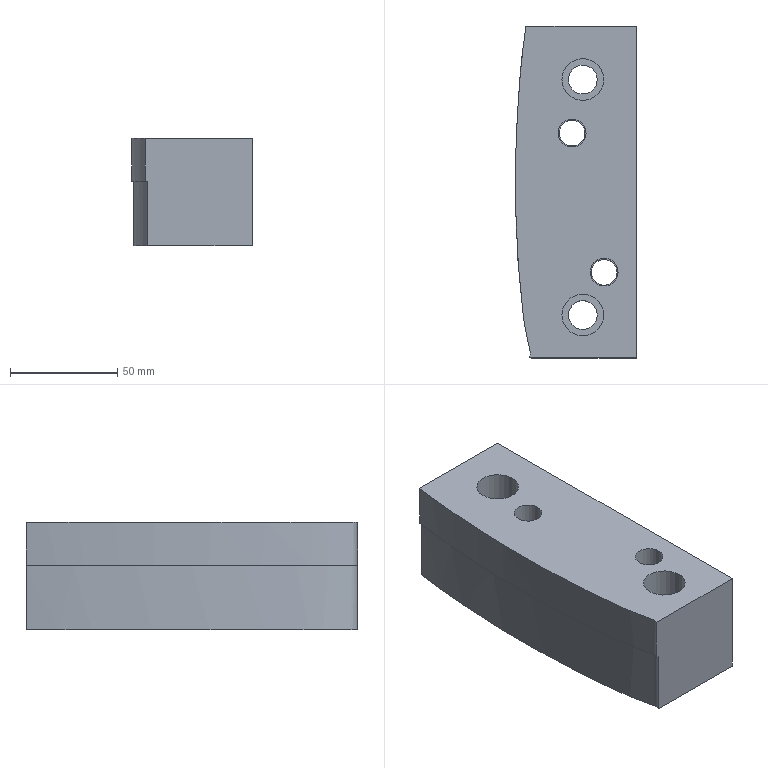Part | NX | features solid 2 | 1 solid | 20 faces | box 56.479 x 155 x 50 mm | volume 388259 mm3 | plane 10 | cylinder 8 | spline 2 | commonest cylinder face diameters 12 x2 13 x2 13.5 x2 19.5 x2
STEP:
#1=CARTESIAN_POINT('',(-411.589,75.,0.));
#2=VERTEX_POINT('',#1);
#3=CARTESIAN_POINT('',(-411.589,75.,-20.));
#4=VERTEX_POINT('',#3);
#5=CARTESIAN_POINT('',(-411.589,75.,-10.));
#6=DIRECTION('',(0.,0.,-1.));
#7=VECTOR('',#6,1000.);
#8=LINE('',#5,#7);
#9=EDGE_CURVE('',#2,#4,#8,.T.);
#10=ORIENTED_EDGE('',*,*,#9,.T.);
#11=CARTESIAN_POINT('',(-410.132,-80.,-20.));
#12=VERTEX_POINT('',#11);
#13=CARTESIAN_POINT('',(-122.997,96.222,-20.));
#14=CARTESIAN_POINT('',(-124.392,96.546,-20.));
#15=CARTESIAN_POINT('',(-126.827,98.157,-20.));
#16=CARTESIAN_POINT('',(-130.155,100.898,-20.));
#17=CARTESIAN_POINT('',(-134.281,102.244,-20.));
#18=CARTESIAN_POINT('',(-139.679,104.141,-20.));
#19=CARTESIAN_POINT('',(-146.371,106.694,-20.));
#20=CARTESIAN_POINT('',(-154.427,109.679,-20.));
#21=CARTESIAN_POINT('',(-161.126,112.208,-20.));
#22=CARTESIAN_POINT('',(-165.815,113.972,-20.));
#23=CARTESIAN_POINT('',(-168.494,114.99,-20.));
#24=CARTESIAN_POINT('',(-171.216,115.884,-20.));
#25=CARTESIAN_POINT('',(-174.721,116.613,-20.));
#26=CARTESIAN_POINT('',(-178.987,117.19,-20.));
#27=CARTESIAN_POINT('',(-183.249,117.724,-20.));
#28=CARTESIAN_POINT('',(-191.788,118.655,-20.));
#29=CARTESIAN_POINT('',(-204.643,119.63,-20.));
#30=CARTESIAN_POINT('',(-218.911,120.84,-20.));
#31=CARTESIAN_POINT('',(-228.851,122.152,-20.));
#32=CARTESIAN_POINT('',(-234.551,122.715,-20.));
#33=CARTESIAN_POINT('',(-238.829,123.073,-20.));
#34=CARTESIAN_POINT('',(-243.12,123.479,-20.));
#35=CARTESIAN_POINT('',(-248.75,124.526,-20.));
#36=CARTESIAN_POINT('',(-255.34,127.421,-20.));
#37=CARTESIAN_POINT('',(-261.873,130.381,-20.));
#38=CARTESIAN_POINT('',(-265.989,133.26,-20.));
#39=CARTESIAN_POINT('',(-268.199,135.082,-20.));
#40=CARTESIAN_POINT('',(-270.393,136.924,-20.));
#41=CARTESIAN_POINT('',(-273.148,139.209,-20.));
#42=CARTESIAN_POINT('',(-277.472,142.965,-20.));
#43=CARTESIAN_POINT('',(-282.708,147.853,-20.));
#44=CARTESIAN_POINT('',(-289.411,153.233,-20.));
#45=CARTESIAN_POINT('',(-298.398,160.336,-20.));
#46=CARTESIAN_POINT('',(-314.207,172.665,-20.));
#47=CARTESIAN_POINT('',(-330.339,184.575,-20.));
#48=CARTESIAN_POINT('',(-343.963,195.04,-20.));
#49=CARTESIAN_POINT('',(-350.855,200.194,-20.));
#50=CARTESIAN_POINT('',(-355.804,205.388,-20.));
#51=CARTESIAN_POINT('',(-359.395,208.889,-20.));
#52=CARTESIAN_POINT('',(-361.592,210.724,-20.));
#53=CARTESIAN_POINT('',(-363.291,212.042,-20.));
#54=CARTESIAN_POINT('',(-364.964,213.384,-20.));
#55=CARTESIAN_POINT('',(-366.621,214.773,-20.));
#56=CARTESIAN_POINT('',(-368.75,215.407,-20.));
#57=CARTESIAN_POINT('',(-370.894,214.756,-20.));
#58=CARTESIAN_POINT('',(-372.124,213.383,-20.));
#59=CARTESIAN_POINT('',(-372.711,212.074,-20.));
#60=CARTESIAN_POINT('',(-373.494,210.073,-20.));
#61=CARTESIAN_POINT('',(-374.087,207.63,-20.));
#62=CARTESIAN_POINT('',(-375.074,204.941,-20.));
#63=CARTESIAN_POINT('',(-375.964,202.22,-20.));
#64=CARTESIAN_POINT('',(-377.061,198.808,-20.));
#65=CARTESIAN_POINT('',(-378.358,194.734,-20.));
#66=CARTESIAN_POINT('',(-379.476,191.261,-20.));
#67=CARTESIAN_POINT('',(-381.61,189.247,-20.));
#68=CARTESIAN_POINT('',(-384.401,188.338,-20.));
#69=CARTESIAN_POINT('',(-387.982,189.153,-20.));
#70=CARTESIAN_POINT('',(-392.089,190.337,-20.));
#71=CARTESIAN_POINT('',(-397.637,191.766,-20.));
#72=CARTESIAN_POINT('',(-402.142,192.907,-20.));
#73=CARTESIAN_POINT('',(-405.767,193.016,-20.));
#74=CARTESIAN_POINT('',(-406.752,192.482,-20.));
#75=CARTESIAN_POINT('',(-407.204,191.679,-20.));
#76=CARTESIAN_POINT('',(-407.355,190.978,-20.));
#77=CARTESIAN_POINT('',(-407.778,189.239,-20.));
#78=CARTESIAN_POINT('',(-409.476,182.099,-20.));
#79=CARTESIAN_POINT('',(-411.921,172.376,-20.));
#80=CARTESIAN_POINT('',(-414.76,162.76,-20.));
#81=CARTESIAN_POINT('',(-416.63,157.346,-20.));
#82=CARTESIAN_POINT('',(-418.178,153.337,-20.));
#83=CARTESIAN_POINT('',(-420.236,149.537,-20.));
#84=CARTESIAN_POINT('',(-423.236,146.416,-20.));
#85=CARTESIAN_POINT('',(-426.787,143.984,-20.));
#86=CARTESIAN_POINT('',(-431.478,140.7,-20.));
#87=CARTESIAN_POINT('',(-437.23,136.434,-20.));
#88=CARTESIAN_POINT('',(-444.283,131.521,-20.));
#89=CARTESIAN_POINT('',(-450.102,127.369,-20.));
#90=CARTESIAN_POINT('',(-454.183,123.24,-20.));
#91=CARTESIAN_POINT('',(-456.026,120.178,-20.));
#92=CARTESIAN_POINT('',(-456.869,117.432,-20.));
#93=CARTESIAN_POINT('',(-457.557,114.647,-20.));
#94=CARTESIAN_POINT('',(-458.426,111.177,-20.));
#95=CARTESIAN_POINT('',(-459.295,107.705,-20.));
#96=CARTESIAN_POINT('',(-460.068,104.944,-20.));
#97=CARTESIAN_POINT('',(-460.556,102.852,-20.));
#98=CARTESIAN_POINT('',(-460.759,100.705,-20.));
#99=CARTESIAN_POINT('',(-460.539,97.842,-20.));
#100=CARTESIAN_POINT('',(-458.816,93.054,-20.));
#101=CARTESIAN_POINT('',(-454.37,88.976,-20.));
#102=CARTESIAN_POINT('',(-449.483,87.695,-20.));
#103=CARTESIAN_POINT('',(-446.657,87.236,-20.));
#104=CARTESIAN_POINT('',(-443.828,86.787,-20.));
#105=CARTESIAN_POINT('',(-440.31,86.125,-20.));
#106=CARTESIAN_POINT('',(-434.679,85.08,-20.));
#107=CARTESIAN_POINT('',(-427.604,83.939,-20.));
#108=CARTESIAN_POINT('',(-420.684,82.057,-20.));
#109=CARTESIAN_POINT('',(-415.851,80.778,-20.));
#110=CARTESIAN_POINT('',(-413.367,80.304,-20.));
#111=CARTESIAN_POINT('',(-412.158,79.475,-20.));
#112=CARTESIAN_POINT('',(-411.532,78.587,-20.));
#113=CARTESIAN_POINT('',(-411.333,77.527,-20.));
#114=CARTESIAN_POINT('',(-411.398,76.071,-20.));
#115=CARTESIAN_POINT('',(-411.844,73.616,-20.));
#116=CARTESIAN_POINT('',(-412.388,68.624,-20.));
#117=CARTESIAN_POINT('',(-413.428,61.542,-20.));
#118=CARTESIAN_POINT('',(-414.451,50.13,-20.));
#119=CARTESIAN_POINT('',(-415.942,30.138,-20.));
#120=CARTESIAN_POINT('',(-416.835,1.497,-20.));
#121=CARTESIAN_POINT('',(-415.947,-27.14,-20.));
#122=CARTESIAN_POINT('',(-414.318,-47.126,-20.));
#123=CARTESIAN_POINT('',(-413.277,-56.375,-20.));
#124=CARTESIAN_POINT('',(-412.75,-60.639,-20.));
#125=CARTESIAN_POINT('',(-412.511,-62.774,-20.));
#126=CARTESIAN_POINT('',(-412.138,-64.888,-20.));
#127=CARTESIAN_POINT('',(-411.199,-69.083,-20.));
#128=CARTESIAN_POINT('',(-410.509,-72.962,-20.));
#129=CARTESIAN_POINT('',(-409.724,-76.453,-20.));
#130=CARTESIAN_POINT('',(-409.446,-77.862,-20.));
#131=CARTESIAN_POINT('',(-409.727,-79.695,-20.));
#132=CARTESIAN_POINT('',(-410.96,-81.089,-20.));
#133=CARTESIAN_POINT('',(-412.257,-81.717,-20.));
#134=CARTESIAN_POINT('',(-414.338,-82.265,-20.));
#135=CARTESIAN_POINT('',(-417.449,-83.095,-20.));
#136=CARTESIAN_POINT('',(-422.943,-84.715,-20.));
#137=CARTESIAN_POINT('',(-429.89,-86.483,-20.));
#138=CARTESIAN_POINT('',(-438.395,-87.724,-20.));
#139=CARTESIAN_POINT('',(-445.478,-88.761,-20.));
#140=CARTESIAN_POINT('',(-451.053,-90.196,-20.));
#141=CARTESIAN_POINT('',(-456.021,-93.16,-20.));
#142=CARTESIAN_POINT('',(-460.459,-99.179,-20.));
#143=CARTESIAN_POINT('',(-460.609,-106.618,-20.));
#144=CARTESIAN_POINT('',(-458.817,-112.069,-20.));
#145=CARTESIAN_POINT('',(-457.691,-116.214,-20.));
#146=CARTESIAN_POINT('',(-456.643,-120.377,-20.));
#147=CARTESIAN_POINT('',(-454.688,-125.83,-20.));
#148=CARTESIAN_POINT('',(-450.288,-129.768,-20.));
#149=CARTESIAN_POINT('',(-446.15,-132.56,-20.));
#150=CARTESIAN_POINT('',(-443.768,-134.151,-20.));
#151=CARTESIAN_POINT('',(-441.987,-135.352,-20.));
#152=CARTESIAN_POINT('',(-440.183,-136.518,-20.));
#153=CARTESIAN_POINT('',(-437.722,-137.982,-20.));
#154=CARTESIAN_POINT('',(-434.578,-139.696,-20.));
#155=CARTESIAN_POINT('',(-431.016,-142.118,-20.));
#156=CARTESIAN_POINT('',(-427.923,-145.11,-20.));
#157=CARTESIAN_POINT('',(-425.28,-147.528,-20.));
#158=CARTESIAN_POINT('',(-422.996,-149.255,-20.));
#159=CARTESIAN_POINT('',(-420.694,-150.963,-20.));
#160=CARTESIAN_POINT('',(-418.103,-153.445,-20.));
#161=CARTESIAN_POINT('',(-414.699,-158.081,-20.));
#162=CARTESIAN_POINT('',(-411.818,-164.69,-20.));
#163=CARTESIAN_POINT('',(-409.69,-173.02,-20.));
#164=CARTESIAN_POINT('',(-407.349,-181.283,-20.));
#165=CARTESIAN_POINT('',(-405.436,-188.189,-20.));
#166=CARTESIAN_POINT('',(-404.277,-192.687,-20.));
#167=CARTESIAN_POINT('',(-403.731,-194.774,-20.));
#168=CARTESIAN_POINT('',(-402.911,-195.983,-20.));
#169=CARTESIAN_POINT('',(-401.476,-196.55,-20.));
#170=CARTESIAN_POINT('',(-400.058,-196.272,-20.));
#171=CARTESIAN_POINT('',(-398.677,-195.897,-20.));
#172=CARTESIAN_POINT('',(-396.258,-195.238,-20.));
#173=CARTESIAN_POINT('',(-392.822,-194.236,-20.));
#174=CARTESIAN_POINT('',(-389.356,-193.338,-20.));
#175=CARTESIAN_POINT('',(-386.595,-192.576,-20.));
#176=CARTESIAN_POINT('',(-383.879,-191.694,-20.));
#177=CARTESIAN_POINT('',(-381.029,-191.005,-20.));
#178=CARTESIAN_POINT('',(-378.195,-191.605,-20.));
#179=CARTESIAN_POINT('',(-375.647,-193.039,-20.));
#180=CARTESIAN_POINT('',(-373.775,-196.061,-20.));
#181=CARTESIAN_POINT('',(-372.459,-200.297,-20.));
#182=CARTESIAN_POINT('',(-370.755,-204.215,-20.));
#183=CARTESIAN_POINT('',(-369.584,-207.601,-20.));
#184=CARTESIAN_POINT('',(-368.811,-210.358,-20.));
#185=CARTESIAN_POINT('',(-368.284,-212.445,-20.));
#186=CARTESIAN_POINT('',(-367.403,-214.035,-20.));
#187=CARTESIAN_POINT('',(-366.332,-215.009,-20.));
#188=CARTESIAN_POINT('',(-364.997,-215.589,-20.));
#189=CARTESIAN_POINT('',(-363.147,-215.431,-20.));
#190=CARTESIAN_POINT('',(-361.272,-214.331,-20.));
#191=CARTESIAN_POINT('',(-359.608,-212.974,-20.));
#192=CARTESIAN_POINT('',(-356.215,-210.34,-20.));
#193=CARTESIAN_POINT('',(-349.028,-204.423,-20.));
#194=CARTESIAN_POINT('',(-337.771,-195.573,-20.));
#195=CARTESIAN_POINT('',(-324.236,-184.984,-20.));
#196=CARTESIAN_POINT('',(-313.055,-176.037,-20.));
#197=CARTESIAN_POINT('',(-304.322,-168.623,-20.));
#198=CARTESIAN_POINT('',(-297.827,-162.998,-20.));
#199=CARTESIAN_POINT('',(-291.244,-157.477,-20.));
#200=CARTESIAN_POINT('',(-284.555,-152.085,-20.));
#201=CARTESIAN_POINT('',(-277.805,-146.768,-20.));
#202=CARTESIAN_POINT('',(-271.113,-141.381,-20.));
#203=CARTESIAN_POINT('',(-264.538,-135.852,-20.));
#204=CARTESIAN_POINT('',(-257.668,-130.656,-20.));
#205=CARTESIAN_POINT('',(-251.187,-127.53,-20.));
#206=CARTESIAN_POINT('',(-245.74,-125.755,-20.));
#207=CARTESIAN_POINT('',(-241.581,-124.657,-20.));
#208=CARTESIAN_POINT('',(-237.367,-123.812,-20.));
#209=CARTESIAN_POINT('',(-231.672,-123.168,-20.));
#210=CARTESIAN_POINT('',(-224.501,-123.191,-20.));
#211=CARTESIAN_POINT('',(-215.929,-122.567,-20.));
#212=CARTESIAN_POINT('',(-208.768,-122.461,-20.));
#213=CARTESIAN_POINT('',(-203.041,-122.532,-20.));
#214=CARTESIAN_POINT('',(-198.743,-122.639,-20.));
#215=CARTESIAN_POINT('',(-194.457,-122.273,-20.));
#216=CARTESIAN_POINT('',(-191.639,-121.752,-20.));
#217=CARTESIAN_POINT('',(-190.231,-121.49,-20.));
#218=B_SPLINE_CURVE_WITH_KNOTS('',3,(#13,#14,#15,#16,#17,#18,#19,#20,#21,#22,#23,#24,#25,#26,#27,#28,#29,#30,#31,#32,#33,#34,#35,#36,#37,#38,#39,#40,#41,#42,#43,#44,#45,#46,#47,#48,#49,#50,#51,#52,#53,#54,#55,#56,#57,#58,#59,#60,#61,#62,#63,#64,#65,#66,#67,#68,#69,#70,#71,#72,#73,#74,#75,#76,#77,#78,#79,#80,#81,#82,#83,#84,#85,#86,#87,#88,#89,#90,#91,#92,#93,#94,#95,#96,#97,#98,#99,#100,#101,#102,#103,#104,#105,#106,#107,#108,#109,#110,#111,#112,#113,#114,#115,#116,#117,#118,#119,#120,#121,#122,#123,#124,#125,#126,#127,#128,#129,#130,#131,#132,#133,#134,#135,#136,#137,#138,#139,#140,#141,#142,#143,#144,#145,#146,#147,#148,#149,#150,#151,#152,#153,#154,#155,#156,#157,#158,#159,#160,#161,#162,#163,#164,#165,#166,#167,#168,#169,#170,#171,#172,#173,#174,#175,#176,#177,#178,#179,#180,#181,#182,#183,#184,#185,#186,#187,#188,#189,#190,#191,#192,#193,#194,#195,#196,#197,#198,#199,#200,#201,#202,#203,#204,#205,#206,#207,#208,#209,#210,#211,#212,#213,#214,#215,#216,#217),.UNSPECIFIED.,.F.,.F.,(4,1,1,1,1,1,1,1,1,1,1,1,1,1,1,1,1,1,1,1,1,1,1,1,1,1,1,1,1,1,1,1,1,1,1,1,1,1,1,1,1,1,1,1,1,1,1,1,1,1,1,1,1,1,1,1,1,1,1,1,1,1,1,1,1,1,1,1,1,1,1,1,1,1,1,1,1,1,1,1,1,1,1,1,1,1,1,1,1,1,1,1,1,1,1,1,1,1,1,1,1,1,1,1,1,1,1,1,1,1,1,1,1,1,1,1,1,1,1,1,1,1,1,1,1,1,1,1,1,1,1,1,1,1,1,1,1,1,1,1,1,1,1,1,1,1,1,1,1,1,1,1,1,1,1,1,1,1,1,1,1,1,1,1,1,1,1,1,1,1,1,1,1,1,1,1,1,1,1,1,1,1,1,1,1,1,1,1,1,1,1,1,1,1,1,1,1,1,1,1,1,1,4),(0.,0.001837,0.003675,0.005512,0.007349,0.01102,0.0147,0.01837,0.02021,0.02113,0.02205,0.02388,0.02572,0.02756,0.0294,0.03675,0.0441,0.04777,0.04961,0.05144,0.05328,0.05512,0.05879,0.06247,0.06431,0.06522,0.06614,0.06798,0.06982,0.07349,0.07717,0.08084,0.08819,0.1029,0.1066,0.1102,0.1139,0.1158,0.1167,0.1176,0.1185,0.1194,0.1203,0.1213,0.1222,0.1226,0.1231,0.1249,0.1259,0.1268,0.1286,0.1304,0.1323,0.1332,0.1341,0.136,0.1378,0.1396,0.1433,0.1438,0.1442,0.1447,0.1449,0.1451,0.147,0.1543,0.158,0.1598,0.1617,0.1635,0.1654,0.1672,0.169,0.1727,0.1764,0.1801,0.1819,0.1837,0.1846,0.1856,0.1874,0.1892,0.1902,0.1911,0.192,0.1929,0.1948,0.1984,0.2003,0.2012,0.2021,0.2039,0.2058,0.2095,0.2131,0.215,0.2159,0.2163,0.2168,0.2173,0.2177,0.2186,0.2205,0.2242,0.2278,0.2352,0.2499,0.2646,0.2719,0.2756,0.2765,0.2774,0.2784,0.2793,0.2829,0.2834,0.2839,0.2848,0.2857,0.2862,0.2866,0.2885,0.2903,0.294,0.2976,0.3013,0.3032,0.305,0.3087,0.3123,0.3142,0.316,0.3179,0.3197,0.3234,0.3252,0.3261,0.327,0.328,0.3289,0.3307,0.3326,0.3344,0.3362,0.3371,0.3381,0.3399,0.3417,0.3454,0.3491,0.3528,0.3564,0.3583,0.3587,0.3592,0.3601,0.3606,0.361,0.3619,0.3638,0.3656,0.3665,0.3675,0.3693,0.3702,0.3711,0.373,0.3748,0.3766,0.3785,0.3794,0.3803,0.3812,0.3817,0.3822,0.3831,0.384,0.3849,0.3858,0.3895,0.3969,0.4042,0.4116,0.4152,0.4189,0.4226,0.4263,0.4299,0.4336,0.4373,0.441,0.4446,0.4465,0.4483,0.4501,0.452,0.4557,0.4593,0.463,0.4648,0.4667,0.4685,0.4704),.UNSPECIFIED.);
#219=EDGE_CURVE('',#4,#12,#218,.T.);
#220=ORIENTED_EDGE('',*,*,#219,.T.);
#221=CARTESIAN_POINT('',(-410.132,-80.,0.));
#222=VERTEX_POINT('',#221);
#223=CARTESIAN_POINT('',(-410.132,-80.,-10.));
#224=DIRECTION('',(0.,0.,-1.));
#225=VECTOR('',#224,1000.);
#226=LINE('',#223,#225);
#227=EDGE_CURVE('',#12,#222,#226,.F.);
#228=ORIENTED_EDGE('',*,*,#227,.T.);
#229=CARTESIAN_POINT('',(-414.415,50.161,0.));
#230=VERTEX_POINT('',#229);
#231=CARTESIAN_POINT('',(-410.132,-80.,0.));
#232=CARTESIAN_POINT('',(-409.767,-79.417,0.));
#233=CARTESIAN_POINT('',(-409.378,-78.066,0.));
#234=CARTESIAN_POINT('',(-409.818,-76.035,0.));
#235=CARTESIAN_POINT('',(-410.254,-74.044,0.));
#236=CARTESIAN_POINT('',(-410.792,-71.367,0.));
#237=CARTESIAN_POINT('',(-411.427,-68.019,0.));
#238=CARTESIAN_POINT('',(-412.367,-64.026,0.));
#239=CARTESIAN_POINT('',(-412.828,-59.963,0.));
#240=CARTESIAN_POINT('',(-413.495,-54.553,0.));
#241=CARTESIAN_POINT('',(-414.212,-47.772,0.));
#242=CARTESIAN_POINT('',(-414.925,-39.623,0.));
#243=CARTESIAN_POINT('',(-415.494,-31.468,0.));
#244=CARTESIAN_POINT('',(-415.935,-23.306,0.));
#245=CARTESIAN_POINT('',(-416.352,-12.416,0.));
#246=CARTESIAN_POINT('',(-416.559,1.22,0.));
#247=CARTESIAN_POINT('',(-416.324,17.565,0.));
#248=CARTESIAN_POINT('',(-415.624,33.879,0.));
#249=CARTESIAN_POINT('',(-414.856,44.736,0.));
#250=CARTESIAN_POINT('',(-414.415,50.161,0.));
#251=B_SPLINE_CURVE_WITH_KNOTS('',3,(#231,#232,#233,#234,#235,#236,#237,#238,#239,#240,#241,#242,#243,#244,#245,#246,#247,#248,#249,#250),.UNSPECIFIED.,.F.,.F.,(4,1,1,1,1,1,1,1,1,1,1,1,1,1,1,1,1,4),(0.03621,0.03826,0.04031,0.04235,0.0444,0.0485,0.0526,0.0567,0.0608,0.06899,0.07719,0.08538,0.09358,0.1018,0.1182,0.1346,0.1509,0.1673),.UNSPECIFIED.);
#252=EDGE_CURVE('',#222,#230,#251,.T.);
#253=ORIENTED_EDGE('',*,*,#252,.T.);
#254=CARTESIAN_POINT('',(-412.908,65.002,0.));
#255=VERTEX_POINT('',#254);
#256=CARTESIAN_POINT('',(-412.908,65.002,0.));
#257=CARTESIAN_POINT('',(-413.561,60.072,0.));
#258=CARTESIAN_POINT('',(-414.012,55.117,0.));
#259=CARTESIAN_POINT('',(-414.415,50.161,0.));
#260=B_SPLINE_CURVE_WITH_KNOTS('',3,(#256,#257,#258,#259),.UNSPECIFIED.,.F.,.F.,(4,4),(0.007482,0.0224),.UNSPECIFIED.);
#261=EDGE_CURVE('',#230,#255,#260,.F.);
#262=ORIENTED_EDGE('',*,*,#261,.T.);
#263=CARTESIAN_POINT('',(-412.908,65.002,0.));
#264=CARTESIAN_POINT('',(-412.687,66.668,0.));
#265=CARTESIAN_POINT('',(-412.241,70.001,0.));
#266=CARTESIAN_POINT('',(-411.857,73.337,0.));
#267=CARTESIAN_POINT('',(-411.589,75.,0.));
#268=B_SPLINE_CURVE_WITH_KNOTS('',3,(#263,#264,#265,#266,#267),.UNSPECIFIED.,.F.,.F.,(4,1,4),(0.06884,0.07387,0.0789),.UNSPECIFIED.);
#269=EDGE_CURVE('',#255,#2,#268,.T.);
#270=ORIENTED_EDGE('',*,*,#269,.T.);
#271=EDGE_LOOP('',(#10,#220,#228,#253,#262,#270));
#272=FACE_BOUND('',#271,.T.);
#273=CARTESIAN_POINT('',(-411.589,75.,0.));
#274=CARTESIAN_POINT('',(-411.589,75.,-20.));
#275=CARTESIAN_POINT('',(-411.846,73.402,0.));
#276=CARTESIAN_POINT('',(-411.846,73.402,-20.));
#277=CARTESIAN_POINT('',(-412.222,70.176,0.));
#278=CARTESIAN_POINT('',(-412.222,70.176,-20.));
#279=CARTESIAN_POINT('',(-412.864,65.347,0.));
#280=CARTESIAN_POINT('',(-412.864,65.347,-20.));
#281=CARTESIAN_POINT('',(-413.491,60.521,0.));
#282=CARTESIAN_POINT('',(-413.491,60.521,-20.));
#283=CARTESIAN_POINT('',(-414.109,54.059,0.));
#284=CARTESIAN_POINT('',(-414.109,54.059,-20.));
#285=CARTESIAN_POINT('',(-414.762,45.97,0.));
#286=CARTESIAN_POINT('',(-414.762,45.97,-20.));
#287=CARTESIAN_POINT('',(-415.66,33.018,0.));
#288=CARTESIAN_POINT('',(-415.66,33.018,-20.));
#289=CARTESIAN_POINT('',(-416.378,16.802,0.));
#290=CARTESIAN_POINT('',(-416.378,16.802,-20.));
#291=CARTESIAN_POINT('',(-416.545,0.5708,0.));
#292=CARTESIAN_POINT('',(-416.545,0.5708,-20.));
#293=CARTESIAN_POINT('',(-416.333,-12.411,0.));
#294=CARTESIAN_POINT('',(-416.333,-12.411,-20.));
#295=CARTESIAN_POINT('',(-415.996,-22.142,0.));
#296=CARTESIAN_POINT('',(-415.996,-22.142,-20.));
#297=CARTESIAN_POINT('',(-415.479,-31.865,0.));
#298=CARTESIAN_POINT('',(-415.479,-31.865,-20.));
#299=CARTESIAN_POINT('',(-414.778,-41.578,0.));
#300=CARTESIAN_POINT('',(-414.778,-41.578,-20.));
#301=CARTESIAN_POINT('',(-414.021,-49.658,0.));
#302=CARTESIAN_POINT('',(-414.021,-49.658,-20.));
#303=CARTESIAN_POINT('',(-413.306,-56.11,0.));
#304=CARTESIAN_POINT('',(-413.306,-56.11,-20.));
#305=CARTESIAN_POINT('',(-412.812,-60.137,0.));
#306=CARTESIAN_POINT('',(-412.812,-60.137,-20.));
#307=CARTESIAN_POINT('',(-412.432,-63.361,0.));
#308=CARTESIAN_POINT('',(-412.432,-63.361,-20.));
#309=CARTESIAN_POINT('',(-411.95,-65.747,0.));
#310=CARTESIAN_POINT('',(-411.95,-65.747,-20.));
#311=CARTESIAN_POINT('',(-411.426,-68.126,0.));
#312=CARTESIAN_POINT('',(-411.426,-68.126,-20.));
#313=CARTESIAN_POINT('',(-410.958,-70.515,0.));
#314=CARTESIAN_POINT('',(-410.958,-70.515,-20.));
#315=CARTESIAN_POINT('',(-410.478,-72.904,0.));
#316=CARTESIAN_POINT('',(-410.478,-72.904,-20.));
#317=CARTESIAN_POINT('',(-410.02,-75.287,0.));
#318=CARTESIAN_POINT('',(-410.02,-75.287,-20.));
#319=CARTESIAN_POINT('',(-409.347,-77.659,0.));
#320=CARTESIAN_POINT('',(-409.347,-77.659,-20.));
#321=CARTESIAN_POINT('',(-409.703,-79.314,0.));
#322=CARTESIAN_POINT('',(-409.703,-79.314,-20.));
#323=CARTESIAN_POINT('',(-410.132,-80.,0.));
#324=CARTESIAN_POINT('',(-410.132,-80.,-20.));
#325=B_SPLINE_SURFACE_WITH_KNOTS('',3,1,((#273,#274),(#275,#276),(#277,#278),(#279,#280),(#281,#282),(#283,#284),(#285,#286),(#287,#288),(#289,#290),(#291,#292),(#293,#294),(#295,#296),(#297,#298),(#299,#300),(#301,#302),(#303,#304),(#305,#306),(#307,#308),(#309,#310),(#311,#312),(#313,#314),(#315,#316),(#317,#318),(#319,#320),(#321,#322),(#323,#324)),.SURF_OF_LINEAR_EXTRUSION.,.F.,.F.,.F.,(4,1,1,1,1,1,1,1,1,1,1,1,1,1,1,1,1,1,1,1,1,1,1,4),(2,2),(0.2183,0.2204,0.2225,0.2246,0.2267,0.2308,0.235,0.2433,0.2517,0.2558,0.26,0.2642,0.2683,0.2725,0.2746,0.2766,0.2777,0.2787,0.2798,0.2808,0.2819,0.2829,0.2839,0.285),(0.,1.),.UNSPECIFIED.);
#326=ADVANCED_FACE('',(#272),#325,.F.);
#327=CARTESIAN_POINT('',(-384.,25.,-50.));
#328=VERTEX_POINT('',#327);
#329=CARTESIAN_POINT('',(-390.,25.,-50.));
#330=DIRECTION('',(0.,0.,1.));
#331=DIRECTION('',(1.,0.,0.));
#332=AXIS2_PLACEMENT_3D('',#329,#330,#331);
#333=CIRCLE('',#332,6.);
#334=EDGE_CURVE('',#328,#328,#333,.T.);
#335=ORIENTED_EDGE('',*,*,#334,.T.);
#336=EDGE_LOOP('',(#335));
#337=FACE_BOUND('',#336,.T.);
#338=CARTESIAN_POINT('',(-369.,-40.,-50.));
#339=VERTEX_POINT('',#338);
#340=CARTESIAN_POINT('',(-375.,-40.,-50.));
#341=DIRECTION('',(0.,0.,1.));
#342=DIRECTION('',(1.,0.,0.));
#343=AXIS2_PLACEMENT_3D('',#340,#341,#342);
#344=CIRCLE('',#343,6.);
#345=EDGE_CURVE('',#339,#339,#344,.T.);
#346=ORIENTED_EDGE('',*,*,#345,.T.);
#347=EDGE_LOOP('',(#346));
#348=FACE_BOUND('',#347,.T.);
#349=CARTESIAN_POINT('',(-378.25,-60.,-50.));
#350=VERTEX_POINT('',#349);
#351=CARTESIAN_POINT('',(-385.,-60.,-50.));
#352=DIRECTION('',(0.,0.,1.));
#353=DIRECTION('',(1.,0.,0.));
#354=AXIS2_PLACEMENT_3D('',#351,#352,#353);
#355=CIRCLE('',#354,6.75);
#356=EDGE_CURVE('',#350,#350,#355,.T.);
#357=ORIENTED_EDGE('',*,*,#356,.T.);
#358=EDGE_LOOP('',(#357));
#359=FACE_BOUND('',#358,.T.);
#360=CARTESIAN_POINT('',(-378.25,50.,-50.));
#361=VERTEX_POINT('',#360);
#362=CARTESIAN_POINT('',(-385.,50.,-50.));
#363=DIRECTION('',(0.,0.,1.));
#364=DIRECTION('',(1.,0.,0.));
#365=AXIS2_PLACEMENT_3D('',#362,#363,#364);
#366=CIRCLE('',#365,6.75);
#367=EDGE_CURVE('',#361,#361,#366,.T.);
#368=ORIENTED_EDGE('',*,*,#367,.T.);
#369=EDGE_LOOP('',(#368));
#370=FACE_BOUND('',#369,.T.);
#371=CARTESIAN_POINT('',(-360.,-80.,-50.));
#372=VERTEX_POINT('',#371);
#373=CARTESIAN_POINT('',(-408.997,-80.,-50.));
#374=VERTEX_POINT('',#373);
#375=CARTESIAN_POINT('',(-405.791,-80.,-50.));
#376=DIRECTION('',(1.,0.,0.));
#377=VECTOR('',#376,1000.);
#378=LINE('',#375,#377);
#379=EDGE_CURVE('',#372,#374,#378,.F.);
#380=ORIENTED_EDGE('',*,*,#379,.T.);
#381=CARTESIAN_POINT('',(-410.577,75.,-50.));
#382=VERTEX_POINT('',#381);
#383=CARTESIAN_POINT('',(-408.997,-80.,-50.));
#384=CARTESIAN_POINT('',(-408.653,-79.251,-50.));
#385=CARTESIAN_POINT('',(-408.378,-77.602,-50.));
#386=CARTESIAN_POINT('',(-409.2,-74.42,-50.));
#387=CARTESIAN_POINT('',(-409.794,-71.216,-50.));
#388=CARTESIAN_POINT('',(-410.43,-68.012,-50.));
#389=CARTESIAN_POINT('',(-410.954,-65.618,-50.));
#390=CARTESIAN_POINT('',(-411.443,-63.221,-50.));
#391=CARTESIAN_POINT('',(-411.821,-59.996,-50.));
#392=CARTESIAN_POINT('',(-412.316,-55.966,-50.));
#393=CARTESIAN_POINT('',(-413.031,-49.512,-50.));
#394=CARTESIAN_POINT('',(-413.787,-41.429,-50.));
#395=CARTESIAN_POINT('',(-414.487,-31.708,-50.));
#396=CARTESIAN_POINT('',(-415.003,-21.97,-50.));
#397=CARTESIAN_POINT('',(-415.336,-12.243,-50.));
#398=CARTESIAN_POINT('',(-415.545,0.7174,-50.));
#399=CARTESIAN_POINT('',(-415.374,16.901,-50.));
#400=CARTESIAN_POINT('',(-414.656,33.064,-50.));
#401=CARTESIAN_POINT('',(-413.758,45.981,-50.));
#402=CARTESIAN_POINT('',(-413.106,54.051,-50.));
#403=CARTESIAN_POINT('',(-412.488,60.503,-50.));
#404=CARTESIAN_POINT('',(-411.855,65.336,-50.));
#405=CARTESIAN_POINT('',(-411.221,70.168,-50.));
#406=CARTESIAN_POINT('',(-410.831,73.391,-50.));
#407=CARTESIAN_POINT('',(-410.577,75.,-50.));
#408=B_SPLINE_CURVE_WITH_KNOTS('',3,(#383,#384,#385,#386,#387,#388,#389,#390,#391,#392,#393,#394,#395,#396,#397,#398,#399,#400,#401,#402,#403,#404,#405,#406,#407),.UNSPECIFIED.,.F.,.F.,(4,1,1,1,1,1,1,1,1,1,1,1,1,1,1,1,1,1,1,1,1,1,4),(0.,0.002435,0.004871,0.009742,0.01218,0.01461,0.01705,0.01948,0.02435,0.02923,0.03897,0.04871,0.05845,0.06819,0.07793,0.09742,0.1169,0.1266,0.1364,0.1413,0.1461,0.151,0.1559),.UNSPECIFIED.);
#409=EDGE_CURVE('',#374,#382,#408,.T.);
#410=ORIENTED_EDGE('',*,*,#409,.T.);
#411=CARTESIAN_POINT('',(-360.,75.,-50.));
#412=VERTEX_POINT('',#411);
#413=CARTESIAN_POINT('',(-415.478,75.,-50.));
#414=DIRECTION('',(1.,0.,0.));
#415=VECTOR('',#414,1000.);
#416=LINE('',#413,#415);
#417=EDGE_CURVE('',#382,#412,#416,.T.);
#418=ORIENTED_EDGE('',*,*,#417,.T.);
#419=CARTESIAN_POINT('',(-360.,35.09,-50.));
#420=DIRECTION('',(0.,1.,0.));
#421=VECTOR('',#420,1000.);
#422=LINE('',#419,#421);
#423=EDGE_CURVE('',#372,#412,#422,.T.);
#424=ORIENTED_EDGE('',*,*,#423,.F.);
#425=EDGE_LOOP('',(#380,#410,#418,#424));
#426=FACE_BOUND('',#425,.T.);
#427=CARTESIAN_POINT('',(-415.478,35.09,-50.));
#428=DIRECTION('',(0.,0.,1.));
#429=DIRECTION('',(1.,0.,0.));
#430=AXIS2_PLACEMENT_3D('',#427,#428,#429);
#431=PLANE('',#430);
#432=ADVANCED_FACE('',(#337,#348,#359,#370,#426),#431,.F.);
#433=ORIENTED_EDGE('',*,*,#423,.T.);
#434=CARTESIAN_POINT('',(-360.,75.,0.));
#435=VERTEX_POINT('',#434);
#436=CARTESIAN_POINT('',(-360.,75.,0.));
#437=DIRECTION('',(0.,0.,-1.));
#438=VECTOR('',#437,1000.);
#439=LINE('',#436,#438);
#440=EDGE_CURVE('',#435,#412,#439,.T.);
#441=ORIENTED_EDGE('',*,*,#440,.F.);
#442=CARTESIAN_POINT('',(-360.,-80.,0.));
#443=VERTEX_POINT('',#442);
#444=CARTESIAN_POINT('',(-360.,-222.,0.));
#445=DIRECTION('',(0.,-1.,0.));
#446=VECTOR('',#445,1000.);
#447=LINE('',#444,#446);
#448=EDGE_CURVE('',#435,#443,#447,.T.);
#449=ORIENTED_EDGE('',*,*,#448,.T.);
#450=CARTESIAN_POINT('',(-360.,-80.,-25.));
#451=DIRECTION('',(0.,0.,-1.));
#452=VECTOR('',#451,1000.);
#453=LINE('',#450,#452);
#454=EDGE_CURVE('',#443,#372,#453,.T.);
#455=ORIENTED_EDGE('',*,*,#454,.T.);
#456=EDGE_LOOP('',(#433,#441,#449,#455));
#457=FACE_BOUND('',#456,.T.);
#458=CARTESIAN_POINT('',(-360.,-125.,0.));
#459=DIRECTION('',(1.,0.,0.));
#460=DIRECTION('',(0.,0.,-1.));
#461=AXIS2_PLACEMENT_3D('',#458,#459,#460);
#462=PLANE('',#461);
#463=ADVANCED_FACE('',(#457),#462,.T.);
#464=CARTESIAN_POINT('',(-396.5,25.,0.));
#465=VERTEX_POINT('',#464);
#466=CARTESIAN_POINT('',(-390.,25.,0.));
#467=DIRECTION('',(0.,0.,-1.));
#468=DIRECTION('',(-1.,0.,0.));
#469=AXIS2_PLACEMENT_3D('',#466,#467,#468);
#470=CIRCLE('',#469,6.5);
#471=EDGE_CURVE('',#465,#465,#470,.T.);
#472=ORIENTED_EDGE('',*,*,#471,.T.);
#473=EDGE_LOOP('',(#472));
#474=FACE_BOUND('',#473,.T.);
#475=CARTESIAN_POINT('',(-381.5,-40.,0.));
#476=VERTEX_POINT('',#475);
#477=CARTESIAN_POINT('',(-375.,-40.,0.));
#478=DIRECTION('',(0.,0.,-1.));
#479=DIRECTION('',(-1.,0.,0.));
#480=AXIS2_PLACEMENT_3D('',#477,#478,#479);
#481=CIRCLE('',#480,6.5);
#482=EDGE_CURVE('',#476,#476,#481,.T.);
#483=ORIENTED_EDGE('',*,*,#482,.T.);
#484=EDGE_LOOP('',(#483));
#485=FACE_BOUND('',#484,.T.);
#486=CARTESIAN_POINT('',(-394.75,-60.,0.));
#487=VERTEX_POINT('',#486);
#488=CARTESIAN_POINT('',(-385.,-60.,0.));
#489=DIRECTION('',(0.,0.,-1.));
#490=DIRECTION('',(-1.,0.,0.));
#491=AXIS2_PLACEMENT_3D('',#488,#489,#490);
#492=CIRCLE('',#491,9.75);
#493=EDGE_CURVE('',#487,#487,#492,.T.);
#494=ORIENTED_EDGE('',*,*,#493,.T.);
#495=EDGE_LOOP('',(#494));
#496=FACE_BOUND('',#495,.T.);
#497=CARTESIAN_POINT('',(-394.75,50.,0.));
#498=VERTEX_POINT('',#497);
#499=CARTESIAN_POINT('',(-385.,50.,0.));
#500=DIRECTION('',(0.,0.,-1.));
#501=DIRECTION('',(-1.,0.,0.));
#502=AXIS2_PLACEMENT_3D('',#499,#500,#501);
#503=CIRCLE('',#502,9.75);
#504=EDGE_CURVE('',#498,#498,#503,.T.);
#505=ORIENTED_EDGE('',*,*,#504,.T.);
#506=EDGE_LOOP('',(#505));
#507=FACE_BOUND('',#506,.T.);
#508=ORIENTED_EDGE('',*,*,#448,.F.);
#509=CARTESIAN_POINT('',(-470.381,75.,0.));
#510=DIRECTION('',(-1.,0.,0.));
#511=VECTOR('',#510,1000.);
#512=LINE('',#509,#511);
#513=EDGE_CURVE('',#435,#2,#512,.T.);
#514=ORIENTED_EDGE('',*,*,#513,.T.);
#515=ORIENTED_EDGE('',*,*,#269,.F.);
#516=ORIENTED_EDGE('',*,*,#261,.F.);
#517=ORIENTED_EDGE('',*,*,#252,.F.);
#518=CARTESIAN_POINT('',(-405.791,-80.,0.));
#519=DIRECTION('',(-1.,0.,0.));
#520=VECTOR('',#519,1000.);
#521=LINE('',#518,#520);
#522=EDGE_CURVE('',#222,#443,#521,.F.);
#523=ORIENTED_EDGE('',*,*,#522,.T.);
#524=EDGE_LOOP('',(#508,#514,#515,#516,#517,#523));
#525=FACE_BOUND('',#524,.T.);
#526=CARTESIAN_POINT('',(-470.381,-222.,0.));
#527=DIRECTION('',(0.,0.,-1.));
#528=DIRECTION('',(-1.,0.,0.));
#529=AXIS2_PLACEMENT_3D('',#526,#527,#528);
#530=PLANE('',#529);
#531=ADVANCED_FACE('',(#474,#485,#496,#507,#525),#530,.F.);
#532=ORIENTED_EDGE('',*,*,#227,.F.);
#533=CARTESIAN_POINT('',(-408.997,-80.,-20.));
#534=VERTEX_POINT('',#533);
#535=CARTESIAN_POINT('',(-405.791,-80.,-20.));
#536=DIRECTION('',(1.,0.,0.));
#537=VECTOR('',#536,1000.);
#538=LINE('',#535,#537);
#539=EDGE_CURVE('',#12,#534,#538,.T.);
#540=ORIENTED_EDGE('',*,*,#539,.T.);
#541=CARTESIAN_POINT('',(-408.997,-80.,-60.));
#542=DIRECTION('',(0.,0.,-1.));
#543=VECTOR('',#542,1000.);
#544=LINE('',#541,#543);
#545=EDGE_CURVE('',#534,#374,#544,.T.);
#546=ORIENTED_EDGE('',*,*,#545,.T.);
#547=ORIENTED_EDGE('',*,*,#379,.F.);
#548=ORIENTED_EDGE('',*,*,#454,.F.);
#549=ORIENTED_EDGE('',*,*,#522,.F.);
#550=EDGE_LOOP('',(#532,#540,#546,#547,#548,#549));
#551=FACE_BOUND('',#550,.T.);
#552=CARTESIAN_POINT('',(-405.791,-80.,-25.));
#553=DIRECTION('',(0.,1.,0.));
#554=DIRECTION('',(0.,0.,1.));
#555=AXIS2_PLACEMENT_3D('',#552,#553,#554);
#556=PLANE('',#555);
#557=ADVANCED_FACE('',(#551),#556,.F.);
#558=CARTESIAN_POINT('',(-410.577,75.,-20.));
#559=VERTEX_POINT('',#558);
#560=CARTESIAN_POINT('',(-410.577,75.,-60.));
#561=DIRECTION('',(0.,0.,-1.));
#562=VECTOR('',#561,1000.);
#563=LINE('',#560,#562);
#564=EDGE_CURVE('',#382,#559,#563,.F.);
#565=ORIENTED_EDGE('',*,*,#564,.T.);
#566=CARTESIAN_POINT('',(-408.459,75.,-20.));
#567=DIRECTION('',(-1.,0.,0.));
#568=VECTOR('',#567,1000.);
#569=LINE('',#566,#568);
#570=EDGE_CURVE('',#559,#4,#569,.T.);
#571=ORIENTED_EDGE('',*,*,#570,.T.);
#572=ORIENTED_EDGE('',*,*,#9,.F.);
#573=ORIENTED_EDGE('',*,*,#513,.F.);
#574=ORIENTED_EDGE('',*,*,#440,.T.);
#575=ORIENTED_EDGE('',*,*,#417,.F.);
#576=EDGE_LOOP('',(#565,#571,#572,#573,#574,#575));
#577=FACE_BOUND('',#576,.T.);
#578=CARTESIAN_POINT('',(-408.459,75.,-25.));
#579=DIRECTION('',(0.,-1.,0.));
#580=DIRECTION('',(0.,0.,-1.));
#581=AXIS2_PLACEMENT_3D('',#578,#579,#580);
#582=PLANE('',#581);
#583=ADVANCED_FACE('',(#577),#582,.F.);
#584=CARTESIAN_POINT('',(-391.75,50.,-15.));
#585=VERTEX_POINT('',#584);
#586=CARTESIAN_POINT('',(-385.,50.,-15.));
#587=DIRECTION('',(0.,0.,-1.));
#588=DIRECTION('',(-1.,0.,0.));
#589=AXIS2_PLACEMENT_3D('',#586,#587,#588);
#590=CIRCLE('',#589,6.75);
#591=EDGE_CURVE('',#585,#585,#590,.T.);
#592=ORIENTED_EDGE('',*,*,#591,.F.);
#593=EDGE_LOOP('',(#592));
#594=FACE_BOUND('',#593,.T.);
#595=ORIENTED_EDGE('',*,*,#367,.F.);
#596=EDGE_LOOP('',(#595));
#597=FACE_BOUND('',#596,.T.);
#598=CARTESIAN_POINT('',(-385.,50.,-100.));
#599=DIRECTION('',(0.,0.,-1.));
#600=DIRECTION('',(-1.,0.,0.));
#601=AXIS2_PLACEMENT_3D('',#598,#599,#600);
#602=CYLINDRICAL_SURFACE('',#601,6.75);
#603=ADVANCED_FACE('',(#594,#597),#602,.F.);
#604=ORIENTED_EDGE('',*,*,#591,.T.);
#605=EDGE_LOOP('',(#604));
#606=FACE_BOUND('',#605,.T.);
#607=CARTESIAN_POINT('',(-394.75,50.,-15.));
#608=VERTEX_POINT('',#607);
#609=CARTESIAN_POINT('',(-385.,50.,-15.));
#610=DIRECTION('',(0.,0.,-1.));
#611=DIRECTION('',(-1.,0.,0.));
#612=AXIS2_PLACEMENT_3D('',#609,#610,#611);
#613=CIRCLE('',#612,9.75);
#614=EDGE_CURVE('',#608,#608,#613,.T.);
#615=ORIENTED_EDGE('',*,*,#614,.F.);
#616=EDGE_LOOP('',(#615));
#617=FACE_BOUND('',#616,.T.);
#618=CARTESIAN_POINT('',(-385.,50.,-15.));
#619=DIRECTION('',(0.,0.,-1.));
#620=DIRECTION('',(-1.,0.,0.));
#621=AXIS2_PLACEMENT_3D('',#618,#619,#620);
#622=PLANE('',#621);
#623=ADVANCED_FACE('',(#606,#617),#622,.F.);
#624=ORIENTED_EDGE('',*,*,#614,.T.);
#625=EDGE_LOOP('',(#624));
#626=FACE_BOUND('',#625,.T.);
#627=ORIENTED_EDGE('',*,*,#504,.F.);
#628=EDGE_LOOP('',(#627));
#629=FACE_BOUND('',#628,.T.);
#630=CARTESIAN_POINT('',(-385.,50.,0.));
#631=DIRECTION('',(0.,0.,-1.));
#632=DIRECTION('',(-1.,0.,0.));
#633=AXIS2_PLACEMENT_3D('',#630,#631,#632);
#634=CYLINDRICAL_SURFACE('',#633,9.75);
#635=ADVANCED_FACE('',(#626,#629),#634,.F.);
#636=CARTESIAN_POINT('',(-391.75,-60.,-15.));
#637=VERTEX_POINT('',#636);
#638=CARTESIAN_POINT('',(-385.,-60.,-15.));
#639=DIRECTION('',(0.,0.,-1.));
#640=DIRECTION('',(-1.,0.,0.));
#641=AXIS2_PLACEMENT_3D('',#638,#639,#640);
#642=CIRCLE('',#641,6.75);
#643=EDGE_CURVE('',#637,#637,#642,.T.);
#644=ORIENTED_EDGE('',*,*,#643,.F.);
#645=EDGE_LOOP('',(#644));
#646=FACE_BOUND('',#645,.T.);
#647=ORIENTED_EDGE('',*,*,#356,.F.);
#648=EDGE_LOOP('',(#647));
#649=FACE_BOUND('',#648,.T.);
#650=CARTESIAN_POINT('',(-385.,-60.,-100.));
#651=DIRECTION('',(0.,0.,-1.));
#652=DIRECTION('',(-1.,0.,0.));
#653=AXIS2_PLACEMENT_3D('',#650,#651,#652);
#654=CYLINDRICAL_SURFACE('',#653,6.75);
#655=ADVANCED_FACE('',(#646,#649),#654,.F.);
#656=ORIENTED_EDGE('',*,*,#643,.T.);
#657=EDGE_LOOP('',(#656));
#658=FACE_BOUND('',#657,.T.);
#659=CARTESIAN_POINT('',(-394.75,-60.,-15.));
#660=VERTEX_POINT('',#659);
#661=CARTESIAN_POINT('',(-385.,-60.,-15.));
#662=DIRECTION('',(0.,0.,-1.));
#663=DIRECTION('',(-1.,0.,0.));
#664=AXIS2_PLACEMENT_3D('',#661,#662,#663);
#665=CIRCLE('',#664,9.75);
#666=EDGE_CURVE('',#660,#660,#665,.T.);
#667=ORIENTED_EDGE('',*,*,#666,.F.);
#668=EDGE_LOOP('',(#667));
#669=FACE_BOUND('',#668,.T.);
#670=CARTESIAN_POINT('',(-385.,-55.,-15.));
#671=DIRECTION('',(0.,0.,-1.));
#672=DIRECTION('',(-1.,0.,0.));
#673=AXIS2_PLACEMENT_3D('',#670,#671,#672);
#674=PLANE('',#673);
#675=ADVANCED_FACE('',(#658,#669),#674,.F.);
#676=ORIENTED_EDGE('',*,*,#666,.T.);
#677=EDGE_LOOP('',(#676));
#678=FACE_BOUND('',#677,.T.);
#679=ORIENTED_EDGE('',*,*,#493,.F.);
#680=EDGE_LOOP('',(#679));
#681=FACE_BOUND('',#680,.T.);
#682=CARTESIAN_POINT('',(-385.,-60.,0.));
#683=DIRECTION('',(0.,0.,-1.));
#684=DIRECTION('',(-1.,0.,0.));
#685=AXIS2_PLACEMENT_3D('',#682,#683,#684);
#686=CYLINDRICAL_SURFACE('',#685,9.75);
#687=ADVANCED_FACE('',(#678,#681),#686,.F.);
#688=CARTESIAN_POINT('',(-381.,-40.,-20.));
#689=VERTEX_POINT('',#688);
#690=CARTESIAN_POINT('',(-375.,-40.,-20.));
#691=DIRECTION('',(0.,0.,-1.));
#692=DIRECTION('',(-1.,0.,0.));
#693=AXIS2_PLACEMENT_3D('',#690,#691,#692);
#694=CIRCLE('',#693,6.);
#695=EDGE_CURVE('',#689,#689,#694,.T.);
#696=ORIENTED_EDGE('',*,*,#695,.F.);
#697=EDGE_LOOP('',(#696));
#698=FACE_BOUND('',#697,.T.);
#699=ORIENTED_EDGE('',*,*,#345,.F.);
#700=EDGE_LOOP('',(#699));
#701=FACE_BOUND('',#700,.T.);
#702=CARTESIAN_POINT('',(-375.,-40.,-100.));
#703=DIRECTION('',(0.,0.,-1.));
#704=DIRECTION('',(-1.,0.,0.));
#705=AXIS2_PLACEMENT_3D('',#702,#703,#704);
#706=CYLINDRICAL_SURFACE('',#705,6.);
#707=ADVANCED_FACE('',(#698,#701),#706,.F.);
#708=ORIENTED_EDGE('',*,*,#695,.T.);
#709=EDGE_LOOP('',(#708));
#710=FACE_BOUND('',#709,.T.);
#711=CARTESIAN_POINT('',(-381.5,-40.,-20.));
#712=VERTEX_POINT('',#711);
#713=CARTESIAN_POINT('',(-375.,-40.,-20.));
#714=DIRECTION('',(0.,0.,-1.));
#715=DIRECTION('',(-1.,0.,0.));
#716=AXIS2_PLACEMENT_3D('',#713,#714,#715);
#717=CIRCLE('',#716,6.5);
#718=EDGE_CURVE('',#712,#712,#717,.T.);
#719=ORIENTED_EDGE('',*,*,#718,.F.);
#720=EDGE_LOOP('',(#719));
#721=FACE_BOUND('',#720,.T.);
#722=CARTESIAN_POINT('',(-370.,-40.,-20.));
#723=DIRECTION('',(0.,0.,-1.));
#724=DIRECTION('',(-1.,0.,0.));
#725=AXIS2_PLACEMENT_3D('',#722,#723,#724);
#726=PLANE('',#725);
#727=ADVANCED_FACE('',(#710,#721),#726,.F.);
#728=ORIENTED_EDGE('',*,*,#718,.T.);
#729=EDGE_LOOP('',(#728));
#730=FACE_BOUND('',#729,.T.);
#731=ORIENTED_EDGE('',*,*,#482,.F.);
#732=EDGE_LOOP('',(#731));
#733=FACE_BOUND('',#732,.T.);
#734=CARTESIAN_POINT('',(-375.,-40.,0.));
#735=DIRECTION('',(0.,0.,-1.));
#736=DIRECTION('',(-1.,0.,0.));
#737=AXIS2_PLACEMENT_3D('',#734,#735,#736);
#738=CYLINDRICAL_SURFACE('',#737,6.5);
#739=ADVANCED_FACE('',(#730,#733),#738,.F.);
#740=CARTESIAN_POINT('',(-396.,25.,-20.));
#741=VERTEX_POINT('',#740);
#742=CARTESIAN_POINT('',(-390.,25.,-20.));
#743=DIRECTION('',(0.,0.,-1.));
#744=DIRECTION('',(-1.,0.,0.));
#745=AXIS2_PLACEMENT_3D('',#742,#743,#744);
#746=CIRCLE('',#745,6.);
#747=EDGE_CURVE('',#741,#741,#746,.T.);
#748=ORIENTED_EDGE('',*,*,#747,.F.);
#749=EDGE_LOOP('',(#748));
#750=FACE_BOUND('',#749,.T.);
#751=ORIENTED_EDGE('',*,*,#334,.F.);
#752=EDGE_LOOP('',(#751));
#753=FACE_BOUND('',#752,.T.);
#754=CARTESIAN_POINT('',(-390.,25.,-100.));
#755=DIRECTION('',(0.,0.,-1.));
#756=DIRECTION('',(-1.,0.,0.));
#757=AXIS2_PLACEMENT_3D('',#754,#755,#756);
#758=CYLINDRICAL_SURFACE('',#757,6.);
#759=ADVANCED_FACE('',(#750,#753),#758,.F.);
#760=ORIENTED_EDGE('',*,*,#747,.T.);
#761=EDGE_LOOP('',(#760));
#762=FACE_BOUND('',#761,.T.);
#763=CARTESIAN_POINT('',(-396.5,25.,-20.));
#764=VERTEX_POINT('',#763);
#765=CARTESIAN_POINT('',(-390.,25.,-20.));
#766=DIRECTION('',(0.,0.,-1.));
#767=DIRECTION('',(-1.,0.,0.));
#768=AXIS2_PLACEMENT_3D('',#765,#766,#767);
#769=CIRCLE('',#768,6.5);
#770=EDGE_CURVE('',#764,#764,#769,.T.);
#771=ORIENTED_EDGE('',*,*,#770,.F.);
#772=EDGE_LOOP('',(#771));
#773=FACE_BOUND('',#772,.T.);
#774=CARTESIAN_POINT('',(-390.,25.,-20.));
#775=DIRECTION('',(0.,0.,-1.));
#776=DIRECTION('',(-1.,0.,0.));
#777=AXIS2_PLACEMENT_3D('',#774,#775,#776);
#778=PLANE('',#777);
#779=ADVANCED_FACE('',(#762,#773),#778,.F.);
#780=ORIENTED_EDGE('',*,*,#770,.T.);
#781=EDGE_LOOP('',(#780));
#782=FACE_BOUND('',#781,.T.);
#783=ORIENTED_EDGE('',*,*,#471,.F.);
#784=EDGE_LOOP('',(#783));
#785=FACE_BOUND('',#784,.T.);
#786=CARTESIAN_POINT('',(-390.,25.,0.));
#787=DIRECTION('',(0.,0.,-1.));
#788=DIRECTION('',(-1.,0.,0.));
#789=AXIS2_PLACEMENT_3D('',#786,#787,#788);
#790=CYLINDRICAL_SURFACE('',#789,6.5);
#791=ADVANCED_FACE('',(#782,#785),#790,.F.);
#792=ORIENTED_EDGE('',*,*,#219,.F.);
#793=ORIENTED_EDGE('',*,*,#570,.F.);
#794=CARTESIAN_POINT('',(-410.577,75.,-20.));
#795=CARTESIAN_POINT('',(-410.705,74.185,-20.));
#796=CARTESIAN_POINT('',(-410.944,72.649,-20.));
#797=CARTESIAN_POINT('',(-411.307,69.417,-20.));
#798=CARTESIAN_POINT('',(-411.852,65.383,-20.));
#799=CARTESIAN_POINT('',(-412.476,60.597,-20.));
#800=CARTESIAN_POINT('',(-413.096,54.18,-20.));
#801=CARTESIAN_POINT('',(-413.748,46.109,-20.));
#802=CARTESIAN_POINT('',(-414.648,33.208,-20.));
#803=CARTESIAN_POINT('',(-415.37,17.051,-20.));
#804=CARTESIAN_POINT('',(-415.545,0.8829,-20.));
#805=CARTESIAN_POINT('',(-415.341,-12.048,-20.));
#806=CARTESIAN_POINT('',(-415.013,-21.741,-20.));
#807=CARTESIAN_POINT('',(-414.504,-31.427,-20.));
#808=CARTESIAN_POINT('',(-413.814,-41.1,-20.));
#809=CARTESIAN_POINT('',(-413.065,-49.149,-20.));
#810=CARTESIAN_POINT('',(-412.366,-55.566,-20.));
#811=CARTESIAN_POINT('',(-411.861,-59.597,-20.));
#812=CARTESIAN_POINT('',(-411.507,-62.787,-20.));
#813=CARTESIAN_POINT('',(-410.92,-65.861,-20.));
#814=CARTESIAN_POINT('',(-410.208,-69.084,-20.));
#815=CARTESIAN_POINT('',(-409.597,-72.255,-20.));
#816=CARTESIAN_POINT('',(-409.19,-74.231,-20.));
#817=CARTESIAN_POINT('',(-408.853,-75.791,-20.));
#818=CARTESIAN_POINT('',(-408.559,-77.021,-20.));
#819=CARTESIAN_POINT('',(-408.511,-78.558,-20.));
#820=CARTESIAN_POINT('',(-408.783,-79.533,-20.));
#821=CARTESIAN_POINT('',(-408.997,-80.,-20.));
#822=B_SPLINE_CURVE_WITH_KNOTS('',3,(#794,#795,#796,#797,#798,#799,#800,#801,#802,#803,#804,#805,#806,#807,#808,#809,#810,#811,#812,#813,#814,#815,#816,#817,#818,#819,#820,#821),.UNSPECIFIED.,.F.,.F.,(4,1,1,1,1,1,1,1,1,1,1,1,1,1,1,1,1,1,1,1,1,1,1,1,1,4),(0.2183,0.2193,0.2204,0.2224,0.2245,0.2266,0.2307,0.2349,0.2432,0.2515,0.2557,0.2598,0.264,0.2681,0.2723,0.2744,0.2765,0.2775,0.2785,0.2806,0.2817,0.2827,0.2832,0.2837,0.2843,0.2848),.UNSPECIFIED.);
#823=EDGE_CURVE('',#559,#534,#822,.T.);
#824=ORIENTED_EDGE('',*,*,#823,.T.);
#825=ORIENTED_EDGE('',*,*,#539,.F.);
#826=EDGE_LOOP('',(#792,#793,#824,#825));
#827=FACE_BOUND('',#826,.T.);
#828=CARTESIAN_POINT('',(-190.231,-121.49,-20.));
#829=DIRECTION('',(0.,0.,1.));
#830=DIRECTION('',(1.,0.,0.));
#831=AXIS2_PLACEMENT_3D('',#828,#829,#830);
#832=PLANE('',#831);
#833=ADVANCED_FACE('',(#827),#832,.F.);
#834=ORIENTED_EDGE('',*,*,#823,.F.);
#835=ORIENTED_EDGE('',*,*,#564,.F.);
#836=ORIENTED_EDGE('',*,*,#409,.F.);
#837=ORIENTED_EDGE('',*,*,#545,.F.);
#838=EDGE_LOOP('',(#834,#835,#836,#837));
#839=FACE_BOUND('',#838,.T.);
#840=CARTESIAN_POINT('',(-410.577,75.,-20.));
#841=CARTESIAN_POINT('',(-410.577,75.,-50.));
#842=CARTESIAN_POINT('',(-410.705,74.185,-20.));
#843=CARTESIAN_POINT('',(-410.705,74.185,-50.));
#844=CARTESIAN_POINT('',(-410.944,72.649,-20.));
#845=CARTESIAN_POINT('',(-410.944,72.649,-50.));
#846=CARTESIAN_POINT('',(-411.307,69.417,-20.));
#847=CARTESIAN_POINT('',(-411.307,69.417,-50.));
#848=CARTESIAN_POINT('',(-411.852,65.383,-20.));
#849=CARTESIAN_POINT('',(-411.852,65.383,-50.));
#850=CARTESIAN_POINT('',(-412.476,60.597,-20.));
#851=CARTESIAN_POINT('',(-412.476,60.597,-50.));
#852=CARTESIAN_POINT('',(-413.096,54.18,-20.));
#853=CARTESIAN_POINT('',(-413.096,54.18,-50.));
#854=CARTESIAN_POINT('',(-413.748,46.109,-20.));
#855=CARTESIAN_POINT('',(-413.748,46.109,-50.));
#856=CARTESIAN_POINT('',(-414.648,33.208,-20.));
#857=CARTESIAN_POINT('',(-414.648,33.208,-50.));
#858=CARTESIAN_POINT('',(-415.37,17.051,-20.));
#859=CARTESIAN_POINT('',(-415.37,17.051,-50.));
#860=CARTESIAN_POINT('',(-415.545,0.8829,-20.));
#861=CARTESIAN_POINT('',(-415.545,0.8829,-50.));
#862=CARTESIAN_POINT('',(-415.341,-12.048,-20.));
#863=CARTESIAN_POINT('',(-415.341,-12.048,-50.));
#864=CARTESIAN_POINT('',(-415.013,-21.741,-20.));
#865=CARTESIAN_POINT('',(-415.013,-21.741,-50.));
#866=CARTESIAN_POINT('',(-414.504,-31.427,-20.));
#867=CARTESIAN_POINT('',(-414.504,-31.427,-50.));
#868=CARTESIAN_POINT('',(-413.814,-41.1,-20.));
#869=CARTESIAN_POINT('',(-413.814,-41.1,-50.));
#870=CARTESIAN_POINT('',(-413.065,-49.149,-20.));
#871=CARTESIAN_POINT('',(-413.065,-49.149,-50.));
#872=CARTESIAN_POINT('',(-412.366,-55.566,-20.));
#873=CARTESIAN_POINT('',(-412.366,-55.566,-50.));
#874=CARTESIAN_POINT('',(-411.861,-59.597,-20.));
#875=CARTESIAN_POINT('',(-411.861,-59.597,-50.));
#876=CARTESIAN_POINT('',(-411.507,-62.787,-20.));
#877=CARTESIAN_POINT('',(-411.507,-62.787,-50.));
#878=CARTESIAN_POINT('',(-410.92,-65.861,-20.));
#879=CARTESIAN_POINT('',(-410.92,-65.861,-50.));
#880=CARTESIAN_POINT('',(-410.208,-69.084,-20.));
#881=CARTESIAN_POINT('',(-410.208,-69.084,-50.));
#882=CARTESIAN_POINT('',(-409.597,-72.255,-20.));
#883=CARTESIAN_POINT('',(-409.597,-72.255,-50.));
#884=CARTESIAN_POINT('',(-409.19,-74.231,-20.));
#885=CARTESIAN_POINT('',(-409.19,-74.231,-50.));
#886=CARTESIAN_POINT('',(-408.853,-75.791,-20.));
#887=CARTESIAN_POINT('',(-408.853,-75.791,-50.));
#888=CARTESIAN_POINT('',(-408.559,-77.021,-20.));
#889=CARTESIAN_POINT('',(-408.559,-77.021,-50.));
#890=CARTESIAN_POINT('',(-408.511,-78.558,-20.));
#891=CARTESIAN_POINT('',(-408.511,-78.558,-50.));
#892=CARTESIAN_POINT('',(-408.783,-79.533,-20.));
#893=CARTESIAN_POINT('',(-408.783,-79.533,-50.));
#894=CARTESIAN_POINT('',(-408.997,-80.,-20.));
#895=CARTESIAN_POINT('',(-408.997,-80.,-50.));
#896=B_SPLINE_SURFACE_WITH_KNOTS('',3,1,((#840,#841),(#842,#843),(#844,#845),(#846,#847),(#848,#849),(#850,#851),(#852,#853),(#854,#855),(#856,#857),(#858,#859),(#860,#861),(#862,#863),(#864,#865),(#866,#867),(#868,#869),(#870,#871),(#872,#873),(#874,#875),(#876,#877),(#878,#879),(#880,#881),(#882,#883),(#884,#885),(#886,#887),(#888,#889),(#890,#891),(#892,#893),(#894,#895)),.SURF_OF_LINEAR_EXTRUSION.,.F.,.F.,.F.,(4,1,1,1,1,1,1,1,1,1,1,1,1,1,1,1,1,1,1,1,1,1,1,1,1,4),(2,2),(0.2183,0.2193,0.2204,0.2224,0.2245,0.2266,0.2307,0.2349,0.2432,0.2515,0.2557,0.2598,0.264,0.2681,0.2723,0.2744,0.2765,0.2775,0.2785,0.2806,0.2817,0.2827,0.2832,0.2837,0.2843,0.2848),(0.,1.),.UNSPECIFIED.);
#897=ADVANCED_FACE('',(#839),#896,.F.);
#898=CLOSED_SHELL('',(#326,#432,#463,#531,#557,#583,#603,#623,#635,#655,#675,#687,#707,#727,#739,#759,#779,#791,#833,#897));
#899=MANIFOLD_SOLID_BREP('',#898);
#900=(LENGTH_UNIT()NAMED_UNIT(*)SI_UNIT(.MILLI.,.METRE.));
#901=UNCERTAINTY_MEASURE_WITH_UNIT(LENGTH_MEASURE(0.0508),#900,'','');
#902=(NAMED_UNIT(*)PLANE_ANGLE_UNIT()SI_UNIT($,.RADIAN.));
#903=(NAMED_UNIT(*)SI_UNIT($,.STERADIAN.)SOLID_ANGLE_UNIT());
#904=(GEOMETRIC_REPRESENTATION_CONTEXT(3)GLOBAL_UNCERTAINTY_ASSIGNED_CONTEXT((#901))GLOBAL_UNIT_ASSIGNED_CONTEXT((#900,#902,#903))REPRESENTATION_CONTEXT('',''));
#905=ADVANCED_BREP_SHAPE_REPRESENTATION('',(#899),#904);